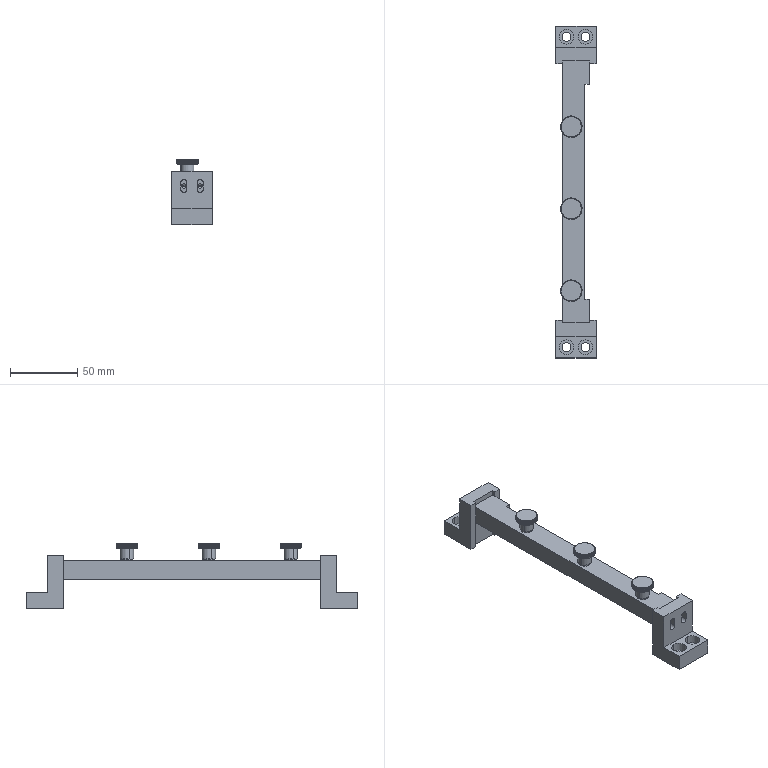Part | SolidWorks | features ReferencePattern 4, LocalLPattern 1 | 9 solids | 537 faces | box 30 x 247 x 49 mm | volume 82433 mm3 | plane 427 | cylinder 76 | cone 34 | commonest cylinder face diameters 8.8 x12 3.3 x8 4 x8 4.5 x8 6.6 x8 11 x8